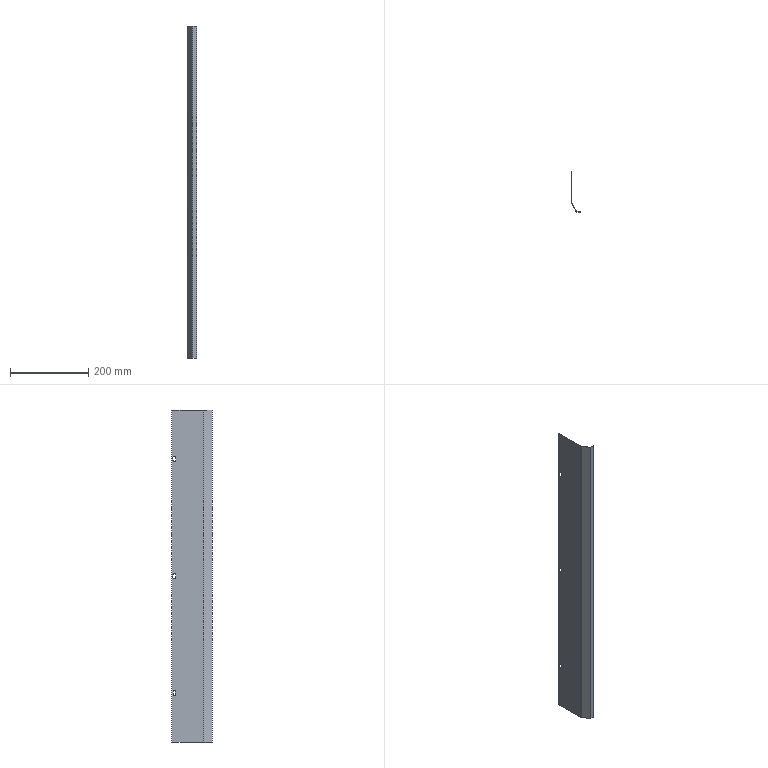Part | SolidWorks | features FlatPattern 1, ICE 1, SMBaseFlange 1, SheetMetal 1 | 1 solid | 37 faces | box 23.5 x 102.651 x 850 mm | volume 98121 mm3 | plane 24 | cylinder 13 | commonest cylinder face diameters 7 x6 6 x3 1 x2 3 x2
STEP:
#1=CARTESIAN_POINT('',(0.,-3.,-296.5));
#2=VERTEX_POINT('',#1);
#3=CARTESIAN_POINT('',(0.,-6.,-293.5));
#4=VERTEX_POINT('',#3);
#5=CARTESIAN_POINT('',(0.,-6.,-296.5));
#6=DIRECTION('',(1.,0.,0.));
#7=DIRECTION('',(0.,1.,0.));
#8=AXIS2_PLACEMENT_3D('',#5,#6,#7);
#9=CIRCLE('',#8,3.);
#10=EDGE_CURVE('',#2,#4,#9,.T.);
#11=ORIENTED_EDGE('',*,*,#10,.T.);
#12=CARTESIAN_POINT('',(-1.,-6.,-293.5));
#13=VERTEX_POINT('',#12);
#14=CARTESIAN_POINT('',(9.,-6.,-293.5));
#15=DIRECTION('',(-1.,0.,0.));
#16=VECTOR('',#15,1000.);
#17=LINE('',#14,#16);
#18=EDGE_CURVE('',#4,#13,#17,.T.);
#19=ORIENTED_EDGE('',*,*,#18,.T.);
#20=CARTESIAN_POINT('',(-1.,-3.,-296.5));
#21=VERTEX_POINT('',#20);
#22=CARTESIAN_POINT('',(-1.,-6.,-296.5));
#23=DIRECTION('',(-1.,0.,0.));
#24=DIRECTION('',(0.,0.,1.));
#25=AXIS2_PLACEMENT_3D('',#22,#23,#24);
#26=CIRCLE('',#25,3.);
#27=EDGE_CURVE('',#13,#21,#26,.T.);
#28=ORIENTED_EDGE('',*,*,#27,.T.);
#29=CARTESIAN_POINT('',(9.,-3.,-296.5));
#30=DIRECTION('',(-1.,0.,0.));
#31=VECTOR('',#30,1000.);
#32=LINE('',#29,#31);
#33=EDGE_CURVE('',#2,#21,#32,.T.);
#34=ORIENTED_EDGE('',*,*,#33,.F.);
#35=EDGE_LOOP('',(#11,#19,#28,#34));
#36=FACE_OUTER_BOUND('',#35,.T.);
#37=CARTESIAN_POINT('',(9.,-6.,-296.5));
#38=DIRECTION('',(-1.,0.,0.));
#39=DIRECTION('',(0.,0.,1.));
#40=AXIS2_PLACEMENT_3D('',#37,#38,#39);
#41=CYLINDRICAL_SURFACE('',#40,3.);
#42=ADVANCED_FACE('',(#36),#41,.F.);
#43=CARTESIAN_POINT('',(0.,-2.5,303.5));
#44=VERTEX_POINT('',#43);
#45=CARTESIAN_POINT('',(0.,-6.,307.));
#46=VERTEX_POINT('',#45);
#47=CARTESIAN_POINT('',(0.,-6.,303.5));
#48=DIRECTION('',(1.,0.,0.));
#49=DIRECTION('',(0.,1.,0.));
#50=AXIS2_PLACEMENT_3D('',#47,#48,#49);
#51=CIRCLE('',#50,3.5);
#52=EDGE_CURVE('',#44,#46,#51,.T.);
#53=ORIENTED_EDGE('',*,*,#52,.T.);
#54=CARTESIAN_POINT('',(-1.,-6.,307.));
#55=VERTEX_POINT('',#54);
#56=CARTESIAN_POINT('',(9.,-6.,307.));
#57=DIRECTION('',(-1.,0.,0.));
#58=VECTOR('',#57,1000.);
#59=LINE('',#56,#58);
#60=EDGE_CURVE('',#46,#55,#59,.T.);
#61=ORIENTED_EDGE('',*,*,#60,.T.);
#62=CARTESIAN_POINT('',(-1.,-2.5,303.5));
#63=VERTEX_POINT('',#62);
#64=CARTESIAN_POINT('',(-1.,-6.,303.5));
#65=DIRECTION('',(-1.,0.,0.));
#66=DIRECTION('',(0.,0.,1.));
#67=AXIS2_PLACEMENT_3D('',#64,#65,#66);
#68=CIRCLE('',#67,3.5);
#69=EDGE_CURVE('',#55,#63,#68,.T.);
#70=ORIENTED_EDGE('',*,*,#69,.T.);
#71=CARTESIAN_POINT('',(9.,-2.5,303.5));
#72=DIRECTION('',(-1.,0.,0.));
#73=VECTOR('',#72,1000.);
#74=LINE('',#71,#73);
#75=EDGE_CURVE('',#44,#63,#74,.T.);
#76=ORIENTED_EDGE('',*,*,#75,.F.);
#77=EDGE_LOOP('',(#53,#61,#70,#76));
#78=FACE_OUTER_BOUND('',#77,.T.);
#79=CARTESIAN_POINT('',(9.,-6.,303.5));
#80=DIRECTION('',(-1.,0.,0.));
#81=DIRECTION('',(0.,0.,1.));
#82=AXIS2_PLACEMENT_3D('',#79,#80,#81);
#83=CYLINDRICAL_SURFACE('',#82,3.5);
#84=ADVANCED_FACE('',(#78),#83,.F.);
#85=CARTESIAN_POINT('',(0.,-2.5,3.5));
#86=VERTEX_POINT('',#85);
#87=CARTESIAN_POINT('',(0.,-6.,7.));
#88=VERTEX_POINT('',#87);
#89=CARTESIAN_POINT('',(0.,-6.,3.5));
#90=DIRECTION('',(1.,0.,0.));
#91=DIRECTION('',(0.,1.,0.));
#92=AXIS2_PLACEMENT_3D('',#89,#90,#91);
#93=CIRCLE('',#92,3.5);
#94=EDGE_CURVE('',#86,#88,#93,.T.);
#95=ORIENTED_EDGE('',*,*,#94,.T.);
#96=CARTESIAN_POINT('',(-1.,-6.,7.));
#97=VERTEX_POINT('',#96);
#98=CARTESIAN_POINT('',(9.,-6.,7.));
#99=DIRECTION('',(-1.,0.,0.));
#100=VECTOR('',#99,1000.);
#101=LINE('',#98,#100);
#102=EDGE_CURVE('',#88,#97,#101,.T.);
#103=ORIENTED_EDGE('',*,*,#102,.T.);
#104=CARTESIAN_POINT('',(-1.,-2.5,3.5));
#105=VERTEX_POINT('',#104);
#106=CARTESIAN_POINT('',(-1.,-6.,3.5));
#107=DIRECTION('',(-1.,0.,0.));
#108=DIRECTION('',(0.,0.,1.));
#109=AXIS2_PLACEMENT_3D('',#106,#107,#108);
#110=CIRCLE('',#109,3.5);
#111=EDGE_CURVE('',#97,#105,#110,.T.);
#112=ORIENTED_EDGE('',*,*,#111,.T.);
#113=CARTESIAN_POINT('',(9.,-2.5,3.5));
#114=DIRECTION('',(-1.,0.,0.));
#115=VECTOR('',#114,1000.);
#116=LINE('',#113,#115);
#117=EDGE_CURVE('',#86,#105,#116,.T.);
#118=ORIENTED_EDGE('',*,*,#117,.F.);
#119=EDGE_LOOP('',(#95,#103,#112,#118));
#120=FACE_OUTER_BOUND('',#119,.T.);
#121=CARTESIAN_POINT('',(9.,-6.,3.5));
#122=DIRECTION('',(-1.,0.,0.));
#123=DIRECTION('',(0.,0.,1.));
#124=AXIS2_PLACEMENT_3D('',#121,#122,#123);
#125=CYLINDRICAL_SURFACE('',#124,3.5);
#126=ADVANCED_FACE('',(#120),#125,.F.);
#127=CARTESIAN_POINT('',(0.06699,-80.116,425.));
#128=VERTEX_POINT('',#127);
#129=CARTESIAN_POINT('',(-0.799,-80.616,425.));
#130=VERTEX_POINT('',#129);
#131=CARTESIAN_POINT('',(0.06699,-80.116,425.));
#132=DIRECTION('',(-0.866,-0.5,0.));
#133=VECTOR('',#132,1000.);
#134=LINE('',#131,#133);
#135=EDGE_CURVE('',#128,#130,#134,.T.);
#136=ORIENTED_EDGE('',*,*,#135,.F.);
#137=CARTESIAN_POINT('',(0.,-79.866,425.));
#138=VERTEX_POINT('',#137);
#139=CARTESIAN_POINT('',(0.5,-79.866,425.));
#140=DIRECTION('',(0.,0.,1.));
#141=DIRECTION('',(-1.,0.,0.));
#142=AXIS2_PLACEMENT_3D('',#139,#140,#141);
#143=CIRCLE('',#142,0.5);
#144=EDGE_CURVE('',#138,#128,#143,.T.);
#145=ORIENTED_EDGE('',*,*,#144,.F.);
#146=CARTESIAN_POINT('',(-1.,-79.866,425.));
#147=VERTEX_POINT('',#146);
#148=CARTESIAN_POINT('',(-1.,-79.866,425.));
#149=DIRECTION('',(1.,0.,0.));
#150=VECTOR('',#149,1000.);
#151=LINE('',#148,#150);
#152=EDGE_CURVE('',#147,#138,#151,.T.);
#153=ORIENTED_EDGE('',*,*,#152,.F.);
#154=CARTESIAN_POINT('',(0.5,-79.866,425.));
#155=DIRECTION('',(0.,0.,1.));
#156=DIRECTION('',(1.,0.,0.));
#157=AXIS2_PLACEMENT_3D('',#154,#155,#156);
#158=CIRCLE('',#157,1.5);
#159=EDGE_CURVE('',#147,#130,#158,.T.);
#160=ORIENTED_EDGE('',*,*,#159,.T.);
#161=EDGE_LOOP('',(#136,#145,#153,#160));
#162=FACE_OUTER_BOUND('',#161,.T.);
#163=CARTESIAN_POINT('',(0.06699,-80.116,425.));
#164=DIRECTION('',(0.,0.,1.));
#165=DIRECTION('',(1.,0.,0.));
#166=AXIS2_PLACEMENT_3D('',#163,#164,#165);
#167=PLANE('',#166);
#168=ADVANCED_FACE('',(#162),#167,.T.);
#169=CARTESIAN_POINT('',(12.356,-101.401,425.));
#170=VERTEX_POINT('',#169);
#171=CARTESIAN_POINT('',(0.,-80.,425.));
#172=DIRECTION('',(0.5,-0.866,0.));
#173=VECTOR('',#172,1000.);
#174=LINE('',#171,#173);
#175=EDGE_CURVE('',#128,#170,#174,.T.);
#176=ORIENTED_EDGE('',*,*,#175,.F.);
#177=ORIENTED_EDGE('',*,*,#135,.T.);
#178=CARTESIAN_POINT('',(11.49,-101.901,425.));
#179=VERTEX_POINT('',#178);
#180=CARTESIAN_POINT('',(-0.866,-80.5,425.));
#181=DIRECTION('',(0.5,-0.866,0.));
#182=VECTOR('',#181,1000.);
#183=LINE('',#180,#182);
#184=EDGE_CURVE('',#130,#179,#183,.T.);
#185=ORIENTED_EDGE('',*,*,#184,.T.);
#186=CARTESIAN_POINT('',(11.49,-101.901,425.));
#187=DIRECTION('',(0.866,0.5,0.));
#188=VECTOR('',#187,1000.);
#189=LINE('',#186,#188);
#190=EDGE_CURVE('',#179,#170,#189,.T.);
#191=ORIENTED_EDGE('',*,*,#190,.T.);
#192=EDGE_LOOP('',(#176,#177,#185,#191));
#193=FACE_OUTER_BOUND('',#192,.T.);
#194=CARTESIAN_POINT('',(-1.,-79.866,425.));
#195=DIRECTION('',(0.,0.,1.));
#196=DIRECTION('',(1.,0.,0.));
#197=AXIS2_PLACEMENT_3D('',#194,#195,#196);
#198=PLANE('',#197);
#199=ADVANCED_FACE('',(#193),#198,.T.);
#200=CARTESIAN_POINT('',(0.,-79.866,-425.));
#201=VERTEX_POINT('',#200);
#202=CARTESIAN_POINT('',(-1.,-79.866,-425.));
#203=VERTEX_POINT('',#202);
#204=CARTESIAN_POINT('',(0.,-79.866,-425.));
#205=DIRECTION('',(-1.,0.,0.));
#206=VECTOR('',#205,1000.);
#207=LINE('',#204,#206);
#208=EDGE_CURVE('',#201,#203,#207,.T.);
#209=ORIENTED_EDGE('',*,*,#208,.F.);
#210=CARTESIAN_POINT('',(0.06699,-80.116,-425.));
#211=VERTEX_POINT('',#210);
#212=CARTESIAN_POINT('',(0.5,-79.866,-425.));
#213=DIRECTION('',(0.,0.,1.));
#214=DIRECTION('',(-1.,0.,0.));
#215=AXIS2_PLACEMENT_3D('',#212,#213,#214);
#216=CIRCLE('',#215,0.5);
#217=EDGE_CURVE('',#201,#211,#216,.T.);
#218=ORIENTED_EDGE('',*,*,#217,.T.);
#219=CARTESIAN_POINT('',(-0.799,-80.616,-425.));
#220=VERTEX_POINT('',#219);
#221=CARTESIAN_POINT('',(-0.799,-80.616,-425.));
#222=DIRECTION('',(0.866,0.5,0.));
#223=VECTOR('',#222,1000.);
#224=LINE('',#221,#223);
#225=EDGE_CURVE('',#220,#211,#224,.T.);
#226=ORIENTED_EDGE('',*,*,#225,.F.);
#227=CARTESIAN_POINT('',(0.5,-79.866,-425.));
#228=DIRECTION('',(0.,0.,1.));
#229=DIRECTION('',(1.,0.,0.));
#230=AXIS2_PLACEMENT_3D('',#227,#228,#229);
#231=CIRCLE('',#230,1.5);
#232=EDGE_CURVE('',#203,#220,#231,.T.);
#233=ORIENTED_EDGE('',*,*,#232,.F.);
#234=EDGE_LOOP('',(#209,#218,#226,#233));
#235=FACE_OUTER_BOUND('',#234,.T.);
#236=CARTESIAN_POINT('',(0.,-79.866,-425.));
#237=DIRECTION('',(0.,0.,-1.));
#238=DIRECTION('',(-1.,0.,0.));
#239=AXIS2_PLACEMENT_3D('',#236,#237,#238);
#240=PLANE('',#239);
#241=ADVANCED_FACE('',(#235),#240,.T.);
#242=CARTESIAN_POINT('',(0.,0.,-425.));
#243=VERTEX_POINT('',#242);
#244=CARTESIAN_POINT('',(0.,0.,-425.));
#245=DIRECTION('',(0.,-1.,0.));
#246=VECTOR('',#245,1000.);
#247=LINE('',#244,#246);
#248=EDGE_CURVE('',#243,#201,#247,.T.);
#249=ORIENTED_EDGE('',*,*,#248,.T.);
#250=ORIENTED_EDGE('',*,*,#208,.T.);
#251=CARTESIAN_POINT('',(-1.,0.,-425.));
#252=VERTEX_POINT('',#251);
#253=CARTESIAN_POINT('',(-1.,0.,-425.));
#254=DIRECTION('',(0.,-1.,0.));
#255=VECTOR('',#254,1000.);
#256=LINE('',#253,#255);
#257=EDGE_CURVE('',#252,#203,#256,.T.);
#258=ORIENTED_EDGE('',*,*,#257,.F.);
#259=CARTESIAN_POINT('',(-1.,0.,-425.));
#260=DIRECTION('',(1.,0.,0.));
#261=VECTOR('',#260,1000.);
#262=LINE('',#259,#261);
#263=EDGE_CURVE('',#252,#243,#262,.T.);
#264=ORIENTED_EDGE('',*,*,#263,.T.);
#265=EDGE_LOOP('',(#249,#250,#258,#264));
#266=FACE_OUTER_BOUND('',#265,.T.);
#267=CARTESIAN_POINT('',(-0.799,-80.616,-425.));
#268=DIRECTION('',(0.,0.,-1.));
#269=DIRECTION('',(-1.,0.,0.));
#270=AXIS2_PLACEMENT_3D('',#267,#268,#269);
#271=PLANE('',#270);
#272=ADVANCED_FACE('',(#266),#271,.T.);
#273=CARTESIAN_POINT('',(12.789,-101.651,425.));
#274=VERTEX_POINT('',#273);
#275=CARTESIAN_POINT('',(12.789,-102.651,425.));
#276=VERTEX_POINT('',#275);
#277=CARTESIAN_POINT('',(12.789,-101.651,425.));
#278=DIRECTION('',(0.,-1.,0.));
#279=VECTOR('',#278,1000.);
#280=LINE('',#277,#279);
#281=EDGE_CURVE('',#274,#276,#280,.T.);
#282=ORIENTED_EDGE('',*,*,#281,.F.);
#283=CARTESIAN_POINT('',(12.789,-101.151,425.));
#284=DIRECTION('',(0.,0.,1.));
#285=DIRECTION('',(-1.,0.,0.));
#286=AXIS2_PLACEMENT_3D('',#283,#284,#285);
#287=CIRCLE('',#286,0.5);
#288=EDGE_CURVE('',#170,#274,#287,.T.);
#289=ORIENTED_EDGE('',*,*,#288,.F.);
#290=ORIENTED_EDGE('',*,*,#190,.F.);
#291=CARTESIAN_POINT('',(12.789,-101.151,425.));
#292=DIRECTION('',(0.,0.,1.));
#293=DIRECTION('',(1.,0.,0.));
#294=AXIS2_PLACEMENT_3D('',#291,#292,#293);
#295=CIRCLE('',#294,1.5);
#296=EDGE_CURVE('',#179,#276,#295,.T.);
#297=ORIENTED_EDGE('',*,*,#296,.T.);
#298=EDGE_LOOP('',(#282,#289,#290,#297));
#299=FACE_OUTER_BOUND('',#298,.T.);
#300=CARTESIAN_POINT('',(12.789,-101.651,425.));
#301=DIRECTION('',(0.,0.,1.));
#302=DIRECTION('',(1.,0.,0.));
#303=AXIS2_PLACEMENT_3D('',#300,#301,#302);
#304=PLANE('',#303);
#305=ADVANCED_FACE('',(#299),#304,.T.);
#306=CARTESIAN_POINT('',(22.5,-101.651,425.));
#307=VERTEX_POINT('',#306);
#308=CARTESIAN_POINT('',(12.5,-101.651,425.));
#309=DIRECTION('',(1.,0.,0.));
#310=VECTOR('',#309,1000.);
#311=LINE('',#308,#310);
#312=EDGE_CURVE('',#274,#307,#311,.T.);
#313=ORIENTED_EDGE('',*,*,#312,.F.);
#314=ORIENTED_EDGE('',*,*,#281,.T.);
#315=CARTESIAN_POINT('',(22.5,-102.651,425.));
#316=VERTEX_POINT('',#315);
#317=CARTESIAN_POINT('',(12.5,-102.651,425.));
#318=DIRECTION('',(1.,0.,0.));
#319=VECTOR('',#318,1000.);
#320=LINE('',#317,#319);
#321=EDGE_CURVE('',#276,#316,#320,.T.);
#322=ORIENTED_EDGE('',*,*,#321,.T.);
#323=CARTESIAN_POINT('',(22.5,-101.651,425.));
#324=DIRECTION('',(0.,-1.,0.));
#325=VECTOR('',#324,1000.);
#326=LINE('',#323,#325);
#327=EDGE_CURVE('',#307,#316,#326,.T.);
#328=ORIENTED_EDGE('',*,*,#327,.F.);
#329=EDGE_LOOP('',(#313,#314,#322,#328));
#330=FACE_OUTER_BOUND('',#329,.T.);
#331=CARTESIAN_POINT('',(11.49,-101.901,425.));
#332=DIRECTION('',(0.,0.,1.));
#333=DIRECTION('',(1.,0.,0.));
#334=AXIS2_PLACEMENT_3D('',#331,#332,#333);
#335=PLANE('',#334);
#336=ADVANCED_FACE('',(#330),#335,.T.);
#337=CARTESIAN_POINT('',(12.356,-101.401,-425.));
#338=VERTEX_POINT('',#337);
#339=CARTESIAN_POINT('',(11.49,-101.901,-425.));
#340=VERTEX_POINT('',#339);
#341=CARTESIAN_POINT('',(12.356,-101.401,-425.));
#342=DIRECTION('',(-0.866,-0.5,0.));
#343=VECTOR('',#342,1000.);
#344=LINE('',#341,#343);
#345=EDGE_CURVE('',#338,#340,#344,.T.);
#346=ORIENTED_EDGE('',*,*,#345,.F.);
#347=CARTESIAN_POINT('',(12.789,-101.651,-425.));
#348=VERTEX_POINT('',#347);
#349=CARTESIAN_POINT('',(12.789,-101.151,-425.));
#350=DIRECTION('',(0.,0.,1.));
#351=DIRECTION('',(-1.,0.,0.));
#352=AXIS2_PLACEMENT_3D('',#349,#350,#351);
#353=CIRCLE('',#352,0.5);
#354=EDGE_CURVE('',#338,#348,#353,.T.);
#355=ORIENTED_EDGE('',*,*,#354,.T.);
#356=CARTESIAN_POINT('',(12.789,-102.651,-425.));
#357=VERTEX_POINT('',#356);
#358=CARTESIAN_POINT('',(12.789,-102.651,-425.));
#359=DIRECTION('',(0.,1.,0.));
#360=VECTOR('',#359,1000.);
#361=LINE('',#358,#360);
#362=EDGE_CURVE('',#357,#348,#361,.T.);
#363=ORIENTED_EDGE('',*,*,#362,.F.);
#364=CARTESIAN_POINT('',(12.789,-101.151,-425.));
#365=DIRECTION('',(0.,0.,1.));
#366=DIRECTION('',(1.,0.,0.));
#367=AXIS2_PLACEMENT_3D('',#364,#365,#366);
#368=CIRCLE('',#367,1.5);
#369=EDGE_CURVE('',#340,#357,#368,.T.);
#370=ORIENTED_EDGE('',*,*,#369,.F.);
#371=EDGE_LOOP('',(#346,#355,#363,#370));
#372=FACE_OUTER_BOUND('',#371,.T.);
#373=CARTESIAN_POINT('',(12.356,-101.401,-425.));
#374=DIRECTION('',(0.,0.,-1.));
#375=DIRECTION('',(-1.,0.,0.));
#376=AXIS2_PLACEMENT_3D('',#373,#374,#375);
#377=PLANE('',#376);
#378=ADVANCED_FACE('',(#372),#377,.T.);
#379=CARTESIAN_POINT('',(0.,-80.,-425.));
#380=DIRECTION('',(0.5,-0.866,0.));
#381=VECTOR('',#380,1000.);
#382=LINE('',#379,#381);
#383=EDGE_CURVE('',#211,#338,#382,.T.);
#384=ORIENTED_EDGE('',*,*,#383,.T.);
#385=ORIENTED_EDGE('',*,*,#345,.T.);
#386=CARTESIAN_POINT('',(-0.866,-80.5,-425.));
#387=DIRECTION('',(0.5,-0.866,0.));
#388=VECTOR('',#387,1000.);
#389=LINE('',#386,#388);
#390=EDGE_CURVE('',#220,#340,#389,.T.);
#391=ORIENTED_EDGE('',*,*,#390,.F.);
#392=ORIENTED_EDGE('',*,*,#225,.T.);
#393=EDGE_LOOP('',(#384,#385,#391,#392));
#394=FACE_OUTER_BOUND('',#393,.T.);
#395=CARTESIAN_POINT('',(12.789,-102.651,-425.));
#396=DIRECTION('',(0.,0.,-1.));
#397=DIRECTION('',(-1.,0.,0.));
#398=AXIS2_PLACEMENT_3D('',#395,#396,#397);
#399=PLANE('',#398);
#400=ADVANCED_FACE('',(#394),#399,.T.);
#401=CARTESIAN_POINT('',(22.5,-102.651,-425.));
#402=VERTEX_POINT('',#401);
#403=CARTESIAN_POINT('',(12.5,-102.651,-425.));
#404=DIRECTION('',(1.,0.,0.));
#405=VECTOR('',#404,1000.);
#406=LINE('',#403,#405);
#407=EDGE_CURVE('',#357,#402,#406,.T.);
#408=ORIENTED_EDGE('',*,*,#407,.T.);
#409=CARTESIAN_POINT('',(22.5,-102.651,425.));
#410=DIRECTION('',(0.,0.,-1.));
#411=VECTOR('',#410,1000.);
#412=LINE('',#409,#411);
#413=EDGE_CURVE('',#316,#402,#412,.T.);
#414=ORIENTED_EDGE('',*,*,#413,.F.);
#415=ORIENTED_EDGE('',*,*,#321,.F.);
#416=CARTESIAN_POINT('',(12.789,-102.651,425.));
#417=DIRECTION('',(0.,0.,-1.));
#418=VECTOR('',#417,1000.);
#419=LINE('',#416,#418);
#420=EDGE_CURVE('',#276,#357,#419,.T.);
#421=ORIENTED_EDGE('',*,*,#420,.T.);
#422=EDGE_LOOP('',(#408,#414,#415,#421));
#423=FACE_OUTER_BOUND('',#422,.T.);
#424=CARTESIAN_POINT('',(12.5,-102.651,425.));
#425=DIRECTION('',(0.,1.,0.));
#426=DIRECTION('',(0.,0.,1.));
#427=AXIS2_PLACEMENT_3D('',#424,#425,#426);
#428=PLANE('',#427);
#429=ADVANCED_FACE('',(#423),#428,.F.);
#430=CARTESIAN_POINT('',(22.5,-101.651,-425.));
#431=VERTEX_POINT('',#430);
#432=CARTESIAN_POINT('',(22.5,-101.651,-425.));
#433=DIRECTION('',(0.,-1.,0.));
#434=VECTOR('',#433,1000.);
#435=LINE('',#432,#434);
#436=EDGE_CURVE('',#431,#402,#435,.T.);
#437=ORIENTED_EDGE('',*,*,#436,.F.);
#438=CARTESIAN_POINT('',(22.5,-101.651,425.));
#439=DIRECTION('',(0.,0.,-1.));
#440=VECTOR('',#439,1000.);
#441=LINE('',#438,#440);
#442=EDGE_CURVE('',#307,#431,#441,.T.);
#443=ORIENTED_EDGE('',*,*,#442,.F.);
#444=ORIENTED_EDGE('',*,*,#327,.T.);
#445=ORIENTED_EDGE('',*,*,#413,.T.);
#446=EDGE_LOOP('',(#437,#443,#444,#445));
#447=FACE_OUTER_BOUND('',#446,.T.);
#448=CARTESIAN_POINT('',(22.5,-101.651,425.));
#449=DIRECTION('',(1.,0.,0.));
#450=DIRECTION('',(0.,0.,-1.));
#451=AXIS2_PLACEMENT_3D('',#448,#449,#450);
#452=PLANE('',#451);
#453=ADVANCED_FACE('',(#447),#452,.T.);
#454=CARTESIAN_POINT('',(12.5,-101.651,-425.));
#455=DIRECTION('',(1.,0.,0.));
#456=VECTOR('',#455,1000.);
#457=LINE('',#454,#456);
#458=EDGE_CURVE('',#348,#431,#457,.T.);
#459=ORIENTED_EDGE('',*,*,#458,.F.);
#460=CARTESIAN_POINT('',(12.789,-101.651,425.));
#461=DIRECTION('',(0.,0.,-1.));
#462=VECTOR('',#461,1000.);
#463=LINE('',#460,#462);
#464=EDGE_CURVE('',#274,#348,#463,.T.);
#465=ORIENTED_EDGE('',*,*,#464,.F.);
#466=ORIENTED_EDGE('',*,*,#312,.T.);
#467=ORIENTED_EDGE('',*,*,#442,.T.);
#468=EDGE_LOOP('',(#459,#465,#466,#467));
#469=FACE_OUTER_BOUND('',#468,.T.);
#470=CARTESIAN_POINT('',(12.5,-101.651,425.));
#471=DIRECTION('',(0.,1.,0.));
#472=DIRECTION('',(0.,0.,1.));
#473=AXIS2_PLACEMENT_3D('',#470,#471,#472);
#474=PLANE('',#473);
#475=ADVANCED_FACE('',(#469),#474,.T.);
#476=ORIENTED_EDGE('',*,*,#354,.F.);
#477=CARTESIAN_POINT('',(12.356,-101.401,425.));
#478=DIRECTION('',(0.,0.,-1.));
#479=VECTOR('',#478,1000.);
#480=LINE('',#477,#479);
#481=EDGE_CURVE('',#170,#338,#480,.T.);
#482=ORIENTED_EDGE('',*,*,#481,.F.);
#483=ORIENTED_EDGE('',*,*,#288,.T.);
#484=ORIENTED_EDGE('',*,*,#464,.T.);
#485=EDGE_LOOP('',(#476,#482,#483,#484));
#486=FACE_OUTER_BOUND('',#485,.T.);
#487=CARTESIAN_POINT('',(12.789,-101.151,425.));
#488=DIRECTION('',(0.,0.,-1.));
#489=DIRECTION('',(-1.,0.,0.));
#490=AXIS2_PLACEMENT_3D('',#487,#488,#489);
#491=CYLINDRICAL_SURFACE('',#490,0.5);
#492=ADVANCED_FACE('',(#486),#491,.F.);
#493=ORIENTED_EDGE('',*,*,#383,.F.);
#494=CARTESIAN_POINT('',(0.06699,-80.116,425.));
#495=DIRECTION('',(0.,0.,-1.));
#496=VECTOR('',#495,1000.);
#497=LINE('',#494,#496);
#498=EDGE_CURVE('',#128,#211,#497,.T.);
#499=ORIENTED_EDGE('',*,*,#498,.F.);
#500=ORIENTED_EDGE('',*,*,#175,.T.);
#501=ORIENTED_EDGE('',*,*,#481,.T.);
#502=EDGE_LOOP('',(#493,#499,#500,#501));
#503=FACE_OUTER_BOUND('',#502,.T.);
#504=CARTESIAN_POINT('',(0.,-80.,425.));
#505=DIRECTION('',(0.866,0.5,0.));
#506=DIRECTION('',(-0.5,0.866,0.));
#507=AXIS2_PLACEMENT_3D('',#504,#505,#506);
#508=PLANE('',#507);
#509=ADVANCED_FACE('',(#503),#508,.T.);
#510=ORIENTED_EDGE('',*,*,#217,.F.);
#511=CARTESIAN_POINT('',(0.,-79.866,425.));
#512=DIRECTION('',(0.,0.,-1.));
#513=VECTOR('',#512,1000.);
#514=LINE('',#511,#513);
#515=EDGE_CURVE('',#138,#201,#514,.T.);
#516=ORIENTED_EDGE('',*,*,#515,.F.);
#517=ORIENTED_EDGE('',*,*,#144,.T.);
#518=ORIENTED_EDGE('',*,*,#498,.T.);
#519=EDGE_LOOP('',(#510,#516,#517,#518));
#520=FACE_OUTER_BOUND('',#519,.T.);
#521=CARTESIAN_POINT('',(0.5,-79.866,425.));
#522=DIRECTION('',(0.,0.,-1.));
#523=DIRECTION('',(-1.,0.,0.));
#524=AXIS2_PLACEMENT_3D('',#521,#522,#523);
#525=CYLINDRICAL_SURFACE('',#524,0.5);
#526=ADVANCED_FACE('',(#520),#525,.F.);
#527=CARTESIAN_POINT('',(0.,-9.,-303.5));
#528=VERTEX_POINT('',#527);
#529=CARTESIAN_POINT('',(0.,-3.,-303.5));
#530=VERTEX_POINT('',#529);
#531=CARTESIAN_POINT('',(0.,-6.,-303.5));
#532=DIRECTION('',(1.,0.,0.));
#533=DIRECTION('',(0.,1.,0.));
#534=AXIS2_PLACEMENT_3D('',#531,#532,#533);
#535=CIRCLE('',#534,3.);
#536=EDGE_CURVE('',#528,#530,#535,.T.);
#537=ORIENTED_EDGE('',*,*,#536,.F.);
#538=CARTESIAN_POINT('',(0.,-9.,-296.5));
#539=VERTEX_POINT('',#538);
#540=CARTESIAN_POINT('',(0.,-9.,425.));
#541=DIRECTION('',(0.,0.,-1.));
#542=VECTOR('',#541,1000.);
#543=LINE('',#540,#542);
#544=EDGE_CURVE('',#539,#528,#543,.T.);
#545=ORIENTED_EDGE('',*,*,#544,.F.);
#546=CARTESIAN_POINT('',(0.,-6.,-296.5));
#547=DIRECTION('',(1.,0.,0.));
#548=DIRECTION('',(0.,1.,0.));
#549=AXIS2_PLACEMENT_3D('',#546,#547,#548);
#550=CIRCLE('',#549,3.);
#551=EDGE_CURVE('',#4,#539,#550,.T.);
#552=ORIENTED_EDGE('',*,*,#551,.F.);
#553=ORIENTED_EDGE('',*,*,#10,.F.);
#554=CARTESIAN_POINT('',(0.,-3.,425.));
#555=DIRECTION('',(0.,0.,1.));
#556=VECTOR('',#555,1000.);
#557=LINE('',#554,#556);
#558=EDGE_CURVE('',#530,#2,#557,.T.);
#559=ORIENTED_EDGE('',*,*,#558,.F.);
#560=EDGE_LOOP('',(#537,#545,#552,#553,#559));
#561=FACE_BOUND('',#560,.T.);
#562=CARTESIAN_POINT('',(0.,-9.5,296.5));
#563=VERTEX_POINT('',#562);
#564=CARTESIAN_POINT('',(0.,-2.5,296.5));
#565=VERTEX_POINT('',#564);
#566=CARTESIAN_POINT('',(0.,-6.,296.5));
#567=DIRECTION('',(1.,0.,0.));
#568=DIRECTION('',(0.,1.,0.));
#569=AXIS2_PLACEMENT_3D('',#566,#567,#568);
#570=CIRCLE('',#569,3.5);
#571=EDGE_CURVE('',#563,#565,#570,.T.);
#572=ORIENTED_EDGE('',*,*,#571,.F.);
#573=CARTESIAN_POINT('',(0.,-9.5,303.5));
#574=VERTEX_POINT('',#573);
#575=CARTESIAN_POINT('',(0.,-9.5,425.));
#576=DIRECTION('',(0.,0.,-1.));
#577=VECTOR('',#576,1000.);
#578=LINE('',#575,#577);
#579=EDGE_CURVE('',#574,#563,#578,.T.);
#580=ORIENTED_EDGE('',*,*,#579,.F.);
#581=CARTESIAN_POINT('',(0.,-6.,303.5));
#582=DIRECTION('',(1.,0.,0.));
#583=DIRECTION('',(0.,1.,0.));
#584=AXIS2_PLACEMENT_3D('',#581,#582,#583);
#585=CIRCLE('',#584,3.5);
#586=EDGE_CURVE('',#46,#574,#585,.T.);
#587=ORIENTED_EDGE('',*,*,#586,.F.);
#588=ORIENTED_EDGE('',*,*,#52,.F.);
#589=CARTESIAN_POINT('',(0.,-2.5,425.));
#590=DIRECTION('',(0.,0.,1.));
#591=VECTOR('',#590,1000.);
#592=LINE('',#589,#591);
#593=EDGE_CURVE('',#565,#44,#592,.T.);
#594=ORIENTED_EDGE('',*,*,#593,.F.);
#595=EDGE_LOOP('',(#572,#580,#587,#588,#594));
#596=FACE_BOUND('',#595,.T.);
#597=CARTESIAN_POINT('',(0.,-9.5,-3.5));
#598=VERTEX_POINT('',#597);
#599=CARTESIAN_POINT('',(0.,-2.5,-3.5));
#600=VERTEX_POINT('',#599);
#601=CARTESIAN_POINT('',(0.,-6.,-3.5));
#602=DIRECTION('',(1.,0.,0.));
#603=DIRECTION('',(0.,1.,0.));
#604=AXIS2_PLACEMENT_3D('',#601,#602,#603);
#605=CIRCLE('',#604,3.5);
#606=EDGE_CURVE('',#598,#600,#605,.T.);
#607=ORIENTED_EDGE('',*,*,#606,.F.);
#608=CARTESIAN_POINT('',(0.,-9.5,3.5));
#609=VERTEX_POINT('',#608);
#610=CARTESIAN_POINT('',(0.,-9.5,425.));
#611=DIRECTION('',(0.,0.,-1.));
#612=VECTOR('',#611,1000.);
#613=LINE('',#610,#612);
#614=EDGE_CURVE('',#609,#598,#613,.T.);
#615=ORIENTED_EDGE('',*,*,#614,.F.);
#616=CARTESIAN_POINT('',(0.,-6.,3.5));
#617=DIRECTION('',(1.,0.,0.));
#618=DIRECTION('',(0.,1.,0.));
#619=AXIS2_PLACEMENT_3D('',#616,#617,#618);
#620=CIRCLE('',#619,3.5);
#621=EDGE_CURVE('',#88,#609,#620,.T.);
#622=ORIENTED_EDGE('',*,*,#621,.F.);
#623=ORIENTED_EDGE('',*,*,#94,.F.);
#624=CARTESIAN_POINT('',(0.,-2.5,425.));
#625=DIRECTION('',(0.,0.,1.));
#626=VECTOR('',#625,1000.);
#627=LINE('',#624,#626);
#628=EDGE_CURVE('',#600,#86,#627,.T.);
#629=ORIENTED_EDGE('',*,*,#628,.F.);
#630=EDGE_LOOP('',(#607,#615,#622,#623,#629));
#631=FACE_BOUND('',#630,.T.);
#632=ORIENTED_EDGE('',*,*,#248,.F.);
#633=CARTESIAN_POINT('',(0.,0.,425.));
#634=VERTEX_POINT('',#633);
#635=CARTESIAN_POINT('',(0.,0.,425.));
#636=DIRECTION('',(0.,0.,-1.));
#637=VECTOR('',#636,1000.);
#638=LINE('',#635,#637);
#639=EDGE_CURVE('',#634,#243,#638,.T.);
#640=ORIENTED_EDGE('',*,*,#639,.F.);
#641=CARTESIAN_POINT('',(0.,0.,425.));
#642=DIRECTION('',(0.,-1.,0.));
#643=VECTOR('',#642,1000.);
#644=LINE('',#641,#643);
#645=EDGE_CURVE('',#634,#138,#644,.T.);
#646=ORIENTED_EDGE('',*,*,#645,.T.);
#647=ORIENTED_EDGE('',*,*,#515,.T.);
#648=EDGE_LOOP('',(#632,#640,#646,#647));
#649=FACE_OUTER_BOUND('',#648,.T.);
#650=CARTESIAN_POINT('',(0.,0.,425.));
#651=DIRECTION('',(1.,0.,0.));
#652=DIRECTION('',(0.,1.,0.));
#653=AXIS2_PLACEMENT_3D('',#650,#651,#652);
#654=PLANE('',#653);
#655=ADVANCED_FACE('',(#561,#596,#631,#649),#654,.T.);
#656=ORIENTED_EDGE('',*,*,#263,.F.);
#657=CARTESIAN_POINT('',(-1.,0.,425.));
#658=VERTEX_POINT('',#657);
#659=CARTESIAN_POINT('',(-1.,0.,425.));
#660=DIRECTION('',(0.,0.,-1.));
#661=VECTOR('',#660,1000.);
#662=LINE('',#659,#661);
#663=EDGE_CURVE('',#658,#252,#662,.T.);
#664=ORIENTED_EDGE('',*,*,#663,.F.);
#665=CARTESIAN_POINT('',(-1.,0.,425.));
#666=DIRECTION('',(1.,0.,0.));
#667=VECTOR('',#666,1000.);
#668=LINE('',#665,#667);
#669=EDGE_CURVE('',#658,#634,#668,.T.);
#670=ORIENTED_EDGE('',*,*,#669,.T.);
#671=ORIENTED_EDGE('',*,*,#639,.T.);
#672=EDGE_LOOP('',(#656,#664,#670,#671));
#673=FACE_OUTER_BOUND('',#672,.T.);
#674=CARTESIAN_POINT('',(-1.,0.,425.));
#675=DIRECTION('',(0.,1.,0.));
#676=DIRECTION('',(-1.,0.,0.));
#677=AXIS2_PLACEMENT_3D('',#674,#675,#676);
#678=PLANE('',#677);
#679=ADVANCED_FACE('',(#673),#678,.T.);
#680=CARTESIAN_POINT('',(-1.,-9.,-303.5));
#681=VERTEX_POINT('',#680);
#682=CARTESIAN_POINT('',(-1.,-9.,-296.5));
#683=VERTEX_POINT('',#682);
#684=CARTESIAN_POINT('',(-1.,-9.,-303.5));
#685=DIRECTION('',(0.,0.,1.));
#686=VECTOR('',#685,1000.);
#687=LINE('',#684,#686);
#688=EDGE_CURVE('',#681,#683,#687,.T.);
#689=ORIENTED_EDGE('',*,*,#688,.F.);
#690=CARTESIAN_POINT('',(-1.,-3.,-303.5));
#691=VERTEX_POINT('',#690);
#692=CARTESIAN_POINT('',(-1.,-6.,-303.5));
#693=DIRECTION('',(-1.,0.,0.));
#694=DIRECTION('',(0.,0.,1.));
#695=AXIS2_PLACEMENT_3D('',#692,#693,#694);
#696=CIRCLE('',#695,3.);
#697=EDGE_CURVE('',#691,#681,#696,.T.);
#698=ORIENTED_EDGE('',*,*,#697,.F.);
#699=CARTESIAN_POINT('',(-1.,-3.,-303.5));
#700=DIRECTION('',(0.,0.,-1.));
#701=VECTOR('',#700,1000.);
#702=LINE('',#699,#701);
#703=EDGE_CURVE('',#21,#691,#702,.T.);
#704=ORIENTED_EDGE('',*,*,#703,.F.);
#705=ORIENTED_EDGE('',*,*,#27,.F.);
#706=CARTESIAN_POINT('',(-1.,-6.,-296.5));
#707=DIRECTION('',(-1.,0.,0.));
#708=DIRECTION('',(0.,0.,1.));
#709=AXIS2_PLACEMENT_3D('',#706,#707,#708);
#710=CIRCLE('',#709,3.);
#711=EDGE_CURVE('',#683,#13,#710,.T.);
#712=ORIENTED_EDGE('',*,*,#711,.F.);
#713=EDGE_LOOP('',(#689,#698,#704,#705,#712));
#714=FACE_BOUND('',#713,.T.);
#715=CARTESIAN_POINT('',(-1.,-9.5,296.5));
#716=VERTEX_POINT('',#715);
#717=CARTESIAN_POINT('',(-1.,-9.5,303.5));
#718=VERTEX_POINT('',#717);
#719=CARTESIAN_POINT('',(-1.,-9.5,296.5));
#720=DIRECTION('',(0.,0.,1.));
#721=VECTOR('',#720,1000.);
#722=LINE('',#719,#721);
#723=EDGE_CURVE('',#716,#718,#722,.T.);
#724=ORIENTED_EDGE('',*,*,#723,.F.);
#725=CARTESIAN_POINT('',(-1.,-2.5,296.5));
#726=VERTEX_POINT('',#725);
#727=CARTESIAN_POINT('',(-1.,-6.,296.5));
#728=DIRECTION('',(-1.,0.,0.));
#729=DIRECTION('',(0.,0.,1.));
#730=AXIS2_PLACEMENT_3D('',#727,#728,#729);
#731=CIRCLE('',#730,3.5);
#732=EDGE_CURVE('',#726,#716,#731,.T.);
#733=ORIENTED_EDGE('',*,*,#732,.F.);
#734=CARTESIAN_POINT('',(-1.,-2.5,296.5));
#735=DIRECTION('',(0.,0.,-1.));
#736=VECTOR('',#735,1000.);
#737=LINE('',#734,#736);
#738=EDGE_CURVE('',#63,#726,#737,.T.);
#739=ORIENTED_EDGE('',*,*,#738,.F.);
#740=ORIENTED_EDGE('',*,*,#69,.F.);
#741=CARTESIAN_POINT('',(-1.,-6.,303.5));
#742=DIRECTION('',(-1.,0.,0.));
#743=DIRECTION('',(0.,0.,1.));
#744=AXIS2_PLACEMENT_3D('',#741,#742,#743);
#745=CIRCLE('',#744,3.5);
#746=EDGE_CURVE('',#718,#55,#745,.T.);
#747=ORIENTED_EDGE('',*,*,#746,.F.);
#748=EDGE_LOOP('',(#724,#733,#739,#740,#747));
#749=FACE_BOUND('',#748,.T.);
#750=CARTESIAN_POINT('',(-1.,-9.5,-3.5));
#751=VERTEX_POINT('',#750);
#752=CARTESIAN_POINT('',(-1.,-9.5,3.5));
#753=VERTEX_POINT('',#752);
#754=CARTESIAN_POINT('',(-1.,-9.5,-3.5));
#755=DIRECTION('',(0.,0.,1.));
#756=VECTOR('',#755,1000.);
#757=LINE('',#754,#756);
#758=EDGE_CURVE('',#751,#753,#757,.T.);
#759=ORIENTED_EDGE('',*,*,#758,.F.);
#760=CARTESIAN_POINT('',(-1.,-2.5,-3.5));
#761=VERTEX_POINT('',#760);
#762=CARTESIAN_POINT('',(-1.,-6.,-3.5));
#763=DIRECTION('',(-1.,0.,0.));
#764=DIRECTION('',(0.,0.,1.));
#765=AXIS2_PLACEMENT_3D('',#762,#763,#764);
#766=CIRCLE('',#765,3.5);
#767=EDGE_CURVE('',#761,#751,#766,.T.);
#768=ORIENTED_EDGE('',*,*,#767,.F.);
#769=CARTESIAN_POINT('',(-1.,-2.5,-3.5));
#770=DIRECTION('',(0.,0.,-1.));
#771=VECTOR('',#770,1000.);
#772=LINE('',#769,#771);
#773=EDGE_CURVE('',#105,#761,#772,.T.);
#774=ORIENTED_EDGE('',*,*,#773,.F.);
#775=ORIENTED_EDGE('',*,*,#111,.F.);
#776=CARTESIAN_POINT('',(-1.,-6.,3.5));
#777=DIRECTION('',(-1.,0.,0.));
#778=DIRECTION('',(0.,0.,1.));
#779=AXIS2_PLACEMENT_3D('',#776,#777,#778);
#780=CIRCLE('',#779,3.5);
#781=EDGE_CURVE('',#753,#97,#780,.T.);
#782=ORIENTED_EDGE('',*,*,#781,.F.);
#783=EDGE_LOOP('',(#759,#768,#774,#775,#782));
#784=FACE_BOUND('',#783,.T.);
#785=ORIENTED_EDGE('',*,*,#257,.T.);
#786=CARTESIAN_POINT('',(-1.,-79.866,425.));
#787=DIRECTION('',(0.,0.,-1.));
#788=VECTOR('',#787,1000.);
#789=LINE('',#786,#788);
#790=EDGE_CURVE('',#147,#203,#789,.T.);
#791=ORIENTED_EDGE('',*,*,#790,.F.);
#792=CARTESIAN_POINT('',(-1.,0.,425.));
#793=DIRECTION('',(0.,-1.,0.));
#794=VECTOR('',#793,1000.);
#795=LINE('',#792,#794);
#796=EDGE_CURVE('',#658,#147,#795,.T.);
#797=ORIENTED_EDGE('',*,*,#796,.F.);
#798=ORIENTED_EDGE('',*,*,#663,.T.);
#799=EDGE_LOOP('',(#785,#791,#797,#798));
#800=FACE_OUTER_BOUND('',#799,.T.);
#801=CARTESIAN_POINT('',(-1.,0.,425.));
#802=DIRECTION('',(1.,0.,0.));
#803=DIRECTION('',(0.,1.,0.));
#804=AXIS2_PLACEMENT_3D('',#801,#802,#803);
#805=PLANE('',#804);
#806=ADVANCED_FACE('',(#714,#749,#784,#800),#805,.F.);
#807=ORIENTED_EDGE('',*,*,#232,.T.);
#808=CARTESIAN_POINT('',(-0.799,-80.616,425.));
#809=DIRECTION('',(0.,0.,-1.));
#810=VECTOR('',#809,1000.);
#811=LINE('',#808,#810);
#812=EDGE_CURVE('',#130,#220,#811,.T.);
#813=ORIENTED_EDGE('',*,*,#812,.F.);
#814=ORIENTED_EDGE('',*,*,#159,.F.);
#815=ORIENTED_EDGE('',*,*,#790,.T.);
#816=EDGE_LOOP('',(#807,#813,#814,#815));
#817=FACE_OUTER_BOUND('',#816,.T.);
#818=CARTESIAN_POINT('',(0.5,-79.866,425.));
#819=DIRECTION('',(0.,0.,-1.));
#820=DIRECTION('',(-1.,0.,0.));
#821=AXIS2_PLACEMENT_3D('',#818,#819,#820);
#822=CYLINDRICAL_SURFACE('',#821,1.5);
#823=ADVANCED_FACE('',(#817),#822,.T.);
#824=ORIENTED_EDGE('',*,*,#390,.T.);
#825=CARTESIAN_POINT('',(11.49,-101.901,425.));
#826=DIRECTION('',(0.,0.,-1.));
#827=VECTOR('',#826,1000.);
#828=LINE('',#825,#827);
#829=EDGE_CURVE('',#179,#340,#828,.T.);
#830=ORIENTED_EDGE('',*,*,#829,.F.);
#831=ORIENTED_EDGE('',*,*,#184,.F.);
#832=ORIENTED_EDGE('',*,*,#812,.T.);
#833=EDGE_LOOP('',(#824,#830,#831,#832));
#834=FACE_OUTER_BOUND('',#833,.T.);
#835=CARTESIAN_POINT('',(-0.866,-80.5,425.));
#836=DIRECTION('',(0.866,0.5,0.));
#837=DIRECTION('',(-0.5,0.866,0.));
#838=AXIS2_PLACEMENT_3D('',#835,#836,#837);
#839=PLANE('',#838);
#840=ADVANCED_FACE('',(#834),#839,.F.);
#841=ORIENTED_EDGE('',*,*,#369,.T.);
#842=ORIENTED_EDGE('',*,*,#420,.F.);
#843=ORIENTED_EDGE('',*,*,#296,.F.);
#844=ORIENTED_EDGE('',*,*,#829,.T.);
#845=EDGE_LOOP('',(#841,#842,#843,#844));
#846=FACE_OUTER_BOUND('',#845,.T.);
#847=CARTESIAN_POINT('',(12.789,-101.151,425.));
#848=DIRECTION('',(0.,0.,-1.));
#849=DIRECTION('',(-1.,0.,0.));
#850=AXIS2_PLACEMENT_3D('',#847,#848,#849);
#851=CYLINDRICAL_SURFACE('',#850,1.5);
#852=ADVANCED_FACE('',(#846),#851,.T.);
#853=ORIENTED_EDGE('',*,*,#796,.T.);
#854=ORIENTED_EDGE('',*,*,#152,.T.);
#855=ORIENTED_EDGE('',*,*,#645,.F.);
#856=ORIENTED_EDGE('',*,*,#669,.F.);
#857=EDGE_LOOP('',(#853,#854,#855,#856));
#858=FACE_OUTER_BOUND('',#857,.T.);
#859=CARTESIAN_POINT('',(12.789,-101.151,425.));
#860=DIRECTION('',(0.,0.,-1.));
#861=DIRECTION('',(-1.,0.,0.));
#862=AXIS2_PLACEMENT_3D('',#859,#860,#861);
#863=PLANE('',#862);
#864=ADVANCED_FACE('',(#858),#863,.F.);
#865=ORIENTED_EDGE('',*,*,#407,.F.);
#866=ORIENTED_EDGE('',*,*,#362,.T.);
#867=ORIENTED_EDGE('',*,*,#458,.T.);
#868=ORIENTED_EDGE('',*,*,#436,.T.);
#869=EDGE_LOOP('',(#865,#866,#867,#868));
#870=FACE_OUTER_BOUND('',#869,.T.);
#871=CARTESIAN_POINT('',(12.789,-101.151,-425.));
#872=DIRECTION('',(0.,0.,-1.));
#873=DIRECTION('',(-1.,0.,0.));
#874=AXIS2_PLACEMENT_3D('',#871,#872,#873);
#875=PLANE('',#874);
#876=ADVANCED_FACE('',(#870),#875,.T.);
#877=ORIENTED_EDGE('',*,*,#606,.T.);
#878=CARTESIAN_POINT('',(9.,-2.5,-3.5));
#879=DIRECTION('',(-1.,0.,0.));
#880=VECTOR('',#879,1000.);
#881=LINE('',#878,#880);
#882=EDGE_CURVE('',#600,#761,#881,.T.);
#883=ORIENTED_EDGE('',*,*,#882,.T.);
#884=ORIENTED_EDGE('',*,*,#767,.T.);
#885=CARTESIAN_POINT('',(9.,-9.5,-3.5));
#886=DIRECTION('',(-1.,0.,0.));
#887=VECTOR('',#886,1000.);
#888=LINE('',#885,#887);
#889=EDGE_CURVE('',#598,#751,#888,.T.);
#890=ORIENTED_EDGE('',*,*,#889,.F.);
#891=EDGE_LOOP('',(#877,#883,#884,#890));
#892=FACE_OUTER_BOUND('',#891,.T.);
#893=CARTESIAN_POINT('',(9.,-6.,-3.5));
#894=DIRECTION('',(-1.,0.,0.));
#895=DIRECTION('',(0.,0.,1.));
#896=AXIS2_PLACEMENT_3D('',#893,#894,#895);
#897=CYLINDRICAL_SURFACE('',#896,3.5);
#898=ADVANCED_FACE('',(#892),#897,.F.);
#899=ORIENTED_EDGE('',*,*,#628,.T.);
#900=ORIENTED_EDGE('',*,*,#117,.T.);
#901=ORIENTED_EDGE('',*,*,#773,.T.);
#902=ORIENTED_EDGE('',*,*,#882,.F.);
#903=EDGE_LOOP('',(#899,#900,#901,#902));
#904=FACE_OUTER_BOUND('',#903,.T.);
#905=CARTESIAN_POINT('',(9.,-2.5,-3.5));
#906=DIRECTION('',(0.,1.,0.));
#907=DIRECTION('',(0.,0.,1.));
#908=AXIS2_PLACEMENT_3D('',#905,#906,#907);
#909=PLANE('',#908);
#910=ADVANCED_FACE('',(#904),#909,.F.);
#911=ORIENTED_EDGE('',*,*,#102,.F.);
#912=ORIENTED_EDGE('',*,*,#621,.T.);
#913=CARTESIAN_POINT('',(9.,-9.5,3.5));
#914=DIRECTION('',(-1.,0.,0.));
#915=VECTOR('',#914,1000.);
#916=LINE('',#913,#915);
#917=EDGE_CURVE('',#609,#753,#916,.T.);
#918=ORIENTED_EDGE('',*,*,#917,.T.);
#919=ORIENTED_EDGE('',*,*,#781,.T.);
#920=EDGE_LOOP('',(#911,#912,#918,#919));
#921=FACE_OUTER_BOUND('',#920,.T.);
#922=CARTESIAN_POINT('',(9.,-6.,3.5));
#923=DIRECTION('',(-1.,0.,0.));
#924=DIRECTION('',(0.,0.,1.));
#925=AXIS2_PLACEMENT_3D('',#922,#923,#924);
#926=CYLINDRICAL_SURFACE('',#925,3.5);
#927=ADVANCED_FACE('',(#921),#926,.F.);
#928=ORIENTED_EDGE('',*,*,#614,.T.);
#929=ORIENTED_EDGE('',*,*,#889,.T.);
#930=ORIENTED_EDGE('',*,*,#758,.T.);
#931=ORIENTED_EDGE('',*,*,#917,.F.);
#932=EDGE_LOOP('',(#928,#929,#930,#931));
#933=FACE_OUTER_BOUND('',#932,.T.);
#934=CARTESIAN_POINT('',(9.,-9.5,-3.5));
#935=DIRECTION('',(0.,-1.,0.));
#936=DIRECTION('',(0.,0.,-1.));
#937=AXIS2_PLACEMENT_3D('',#934,#935,#936);
#938=PLANE('',#937);
#939=ADVANCED_FACE('',(#933),#938,.F.);
#940=ORIENTED_EDGE('',*,*,#571,.T.);
#941=CARTESIAN_POINT('',(9.,-2.5,296.5));
#942=DIRECTION('',(-1.,0.,0.));
#943=VECTOR('',#942,1000.);
#944=LINE('',#941,#943);
#945=EDGE_CURVE('',#565,#726,#944,.T.);
#946=ORIENTED_EDGE('',*,*,#945,.T.);
#947=ORIENTED_EDGE('',*,*,#732,.T.);
#948=CARTESIAN_POINT('',(9.,-9.5,296.5));
#949=DIRECTION('',(-1.,0.,0.));
#950=VECTOR('',#949,1000.);
#951=LINE('',#948,#950);
#952=EDGE_CURVE('',#563,#716,#951,.T.);
#953=ORIENTED_EDGE('',*,*,#952,.F.);
#954=EDGE_LOOP('',(#940,#946,#947,#953));
#955=FACE_OUTER_BOUND('',#954,.T.);
#956=CARTESIAN_POINT('',(9.,-6.,296.5));
#957=DIRECTION('',(-1.,0.,0.));
#958=DIRECTION('',(0.,0.,1.));
#959=AXIS2_PLACEMENT_3D('',#956,#957,#958);
#960=CYLINDRICAL_SURFACE('',#959,3.5);
#961=ADVANCED_FACE('',(#955),#960,.F.);
#962=ORIENTED_EDGE('',*,*,#593,.T.);
#963=ORIENTED_EDGE('',*,*,#75,.T.);
#964=ORIENTED_EDGE('',*,*,#738,.T.);
#965=ORIENTED_EDGE('',*,*,#945,.F.);
#966=EDGE_LOOP('',(#962,#963,#964,#965));
#967=FACE_OUTER_BOUND('',#966,.T.);
#968=CARTESIAN_POINT('',(9.,-2.5,296.5));
#969=DIRECTION('',(0.,1.,0.));
#970=DIRECTION('',(0.,0.,1.));
#971=AXIS2_PLACEMENT_3D('',#968,#969,#970);
#972=PLANE('',#971);
#973=ADVANCED_FACE('',(#967),#972,.F.);
#974=ORIENTED_EDGE('',*,*,#60,.F.);
#975=ORIENTED_EDGE('',*,*,#586,.T.);
#976=CARTESIAN_POINT('',(9.,-9.5,303.5));
#977=DIRECTION('',(-1.,0.,0.));
#978=VECTOR('',#977,1000.);
#979=LINE('',#976,#978);
#980=EDGE_CURVE('',#574,#718,#979,.T.);
#981=ORIENTED_EDGE('',*,*,#980,.T.);
#982=ORIENTED_EDGE('',*,*,#746,.T.);
#983=EDGE_LOOP('',(#974,#975,#981,#982));
#984=FACE_OUTER_BOUND('',#983,.T.);
#985=CARTESIAN_POINT('',(9.,-6.,303.5));
#986=DIRECTION('',(-1.,0.,0.));
#987=DIRECTION('',(0.,0.,1.));
#988=AXIS2_PLACEMENT_3D('',#985,#986,#987);
#989=CYLINDRICAL_SURFACE('',#988,3.5);
#990=ADVANCED_FACE('',(#984),#989,.F.);
#991=ORIENTED_EDGE('',*,*,#579,.T.);
#992=ORIENTED_EDGE('',*,*,#952,.T.);
#993=ORIENTED_EDGE('',*,*,#723,.T.);
#994=ORIENTED_EDGE('',*,*,#980,.F.);
#995=EDGE_LOOP('',(#991,#992,#993,#994));
#996=FACE_OUTER_BOUND('',#995,.T.);
#997=CARTESIAN_POINT('',(9.,-9.5,296.5));
#998=DIRECTION('',(0.,-1.,0.));
#999=DIRECTION('',(0.,0.,-1.));
#1000=AXIS2_PLACEMENT_3D('',#997,#998,#999);
#1001=PLANE('',#1000);
#1002=ADVANCED_FACE('',(#996),#1001,.F.);
#1003=ORIENTED_EDGE('',*,*,#536,.T.);
#1004=CARTESIAN_POINT('',(9.,-3.,-303.5));
#1005=DIRECTION('',(-1.,0.,0.));
#1006=VECTOR('',#1005,1000.);
#1007=LINE('',#1004,#1006);
#1008=EDGE_CURVE('',#530,#691,#1007,.T.);
#1009=ORIENTED_EDGE('',*,*,#1008,.T.);
#1010=ORIENTED_EDGE('',*,*,#697,.T.);
#1011=CARTESIAN_POINT('',(9.,-9.,-303.5));
#1012=DIRECTION('',(-1.,0.,0.));
#1013=VECTOR('',#1012,1000.);
#1014=LINE('',#1011,#1013);
#1015=EDGE_CURVE('',#528,#681,#1014,.T.);
#1016=ORIENTED_EDGE('',*,*,#1015,.F.);
#1017=EDGE_LOOP('',(#1003,#1009,#1010,#1016));
#1018=FACE_OUTER_BOUND('',#1017,.T.);
#1019=CARTESIAN_POINT('',(9.,-6.,-303.5));
#1020=DIRECTION('',(-1.,0.,0.));
#1021=DIRECTION('',(0.,0.,1.));
#1022=AXIS2_PLACEMENT_3D('',#1019,#1020,#1021);
#1023=CYLINDRICAL_SURFACE('',#1022,3.);
#1024=ADVANCED_FACE('',(#1018),#1023,.F.);
#1025=ORIENTED_EDGE('',*,*,#558,.T.);
#1026=ORIENTED_EDGE('',*,*,#33,.T.);
#1027=ORIENTED_EDGE('',*,*,#703,.T.);
#1028=ORIENTED_EDGE('',*,*,#1008,.F.);
#1029=EDGE_LOOP('',(#1025,#1026,#1027,#1028));
#1030=FACE_OUTER_BOUND('',#1029,.T.);
#1031=CARTESIAN_POINT('',(9.,-3.,-303.5));
#1032=DIRECTION('',(0.,1.,0.));
#1033=DIRECTION('',(0.,0.,1.));
#1034=AXIS2_PLACEMENT_3D('',#1031,#1032,#1033);
#1035=PLANE('',#1034);
#1036=ADVANCED_FACE('',(#1030),#1035,.F.);
#1037=ORIENTED_EDGE('',*,*,#18,.F.);
#1038=ORIENTED_EDGE('',*,*,#551,.T.);
#1039=CARTESIAN_POINT('',(9.,-9.,-296.5));
#1040=DIRECTION('',(-1.,0.,0.));
#1041=VECTOR('',#1040,1000.);
#1042=LINE('',#1039,#1041);
#1043=EDGE_CURVE('',#539,#683,#1042,.T.);
#1044=ORIENTED_EDGE('',*,*,#1043,.T.);
#1045=ORIENTED_EDGE('',*,*,#711,.T.);
#1046=EDGE_LOOP('',(#1037,#1038,#1044,#1045));
#1047=FACE_OUTER_BOUND('',#1046,.T.);
#1048=CARTESIAN_POINT('',(9.,-6.,-296.5));
#1049=DIRECTION('',(-1.,0.,0.));
#1050=DIRECTION('',(0.,0.,1.));
#1051=AXIS2_PLACEMENT_3D('',#1048,#1049,#1050);
#1052=CYLINDRICAL_SURFACE('',#1051,3.);
#1053=ADVANCED_FACE('',(#1047),#1052,.F.);
#1054=ORIENTED_EDGE('',*,*,#544,.T.);
#1055=ORIENTED_EDGE('',*,*,#1015,.T.);
#1056=ORIENTED_EDGE('',*,*,#688,.T.);
#1057=ORIENTED_EDGE('',*,*,#1043,.F.);
#1058=EDGE_LOOP('',(#1054,#1055,#1056,#1057));
#1059=FACE_OUTER_BOUND('',#1058,.T.);
#1060=CARTESIAN_POINT('',(9.,-9.,-303.5));
#1061=DIRECTION('',(0.,-1.,0.));
#1062=DIRECTION('',(0.,0.,-1.));
#1063=AXIS2_PLACEMENT_3D('',#1060,#1061,#1062);
#1064=PLANE('',#1063);
#1065=ADVANCED_FACE('',(#1059),#1064,.F.);
#1066=CLOSED_SHELL('',(#42,#84,#126,#168,#199,#241,#272,#305,#336,#378,#400,#429,#453,#475,#492,#509,#526,#655,#679,#806,#823,#840,#852,#864,#876,#898,#910,#927,#939,#961,#973,#990,#1002,#1024,#1036,#1053,#1065));
#1067=MANIFOLD_SOLID_BREP('',#1066);
#1068=CARTESIAN_POINT('',(0.,0.,0.));
#1069=DIRECTION('',(0.,0.,1.));
#1070=DIRECTION('',(1.,0.,0.));
#1071=AXIS2_PLACEMENT_3D('',#1068,#1069,#1070);
#1072=(LENGTH_UNIT()NAMED_UNIT(*)SI_UNIT(.MILLI.,.METRE.));
#1073=UNCERTAINTY_MEASURE_WITH_UNIT(LENGTH_MEASURE(0.00001),#1072,'','');
#1074=(NAMED_UNIT(*)PLANE_ANGLE_UNIT()SI_UNIT($,.RADIAN.));
#1075=(NAMED_UNIT(*)SI_UNIT($,.STERADIAN.)SOLID_ANGLE_UNIT());
#1076=(GEOMETRIC_REPRESENTATION_CONTEXT(3)GLOBAL_UNCERTAINTY_ASSIGNED_CONTEXT((#1073))GLOBAL_UNIT_ASSIGNED_CONTEXT((#1072,#1074,#1075))REPRESENTATION_CONTEXT('',''));
#1077=ADVANCED_BREP_SHAPE_REPRESENTATION('',(#1067,#1071),#1076);